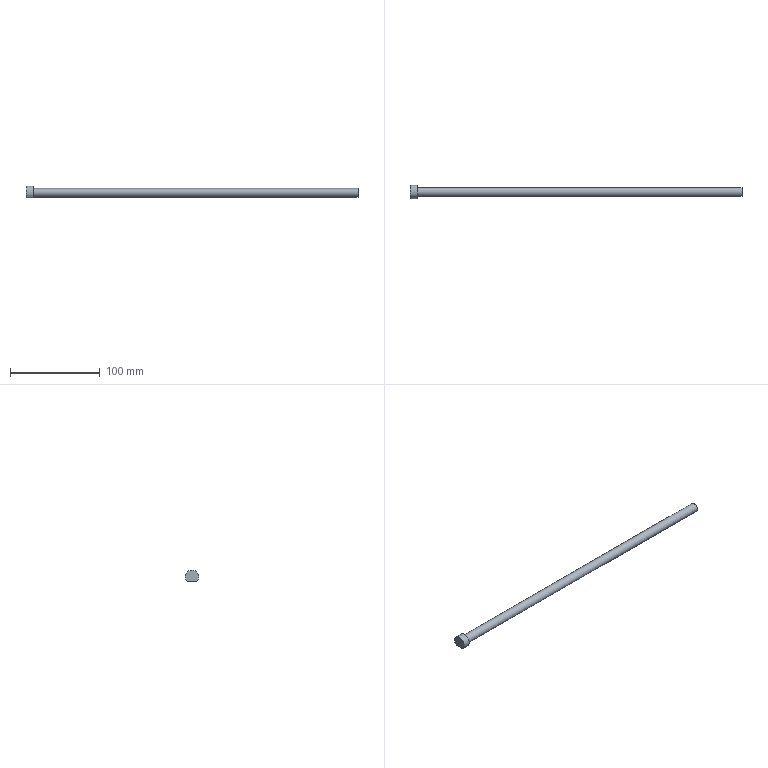Part | STEP file | solid 46 | 1 solid | 6 faces | box 370 x 15 x 13 mm | volume 29733 mm3 | plane 4 | cylinder 2 | commonest cylinder face diameters 10 x1 15 x1